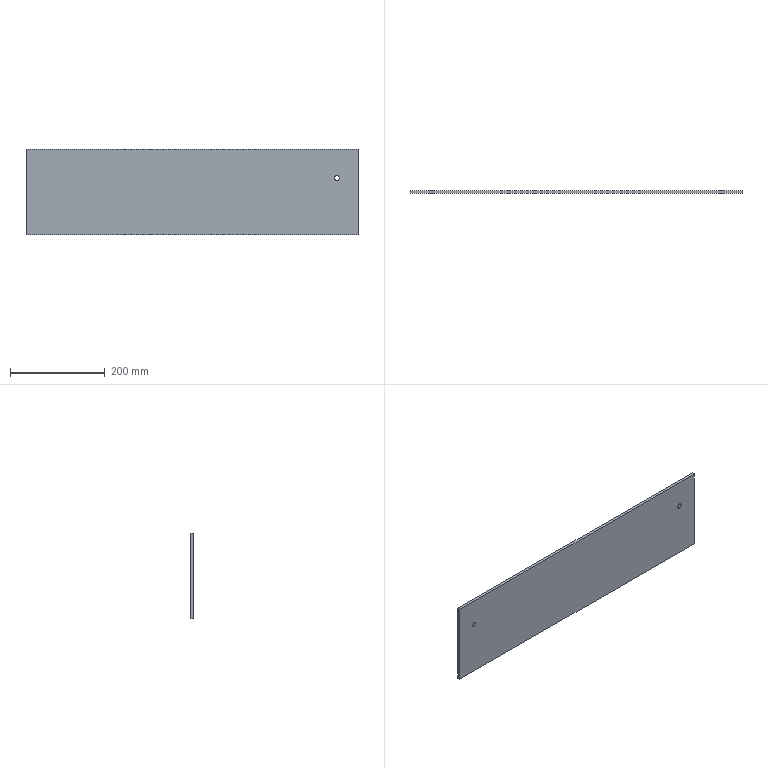Part | SolidWorks | features Cut 2, FlatPattern 1, SMBaseFlange 1, SheetMetal 1 | 1 solid | 11 faces | box 700 x 6 x 180 mm | volume 755105 mm3 | plane 7 | cylinder 4 | commonest cylinder face diameters 10 x4
STEP:
#1=CARTESIAN_POINT('',(48.5,-5.4,-60.5));
#2=VERTEX_POINT('',#1);
#3=CARTESIAN_POINT('',(38.5,-5.4,-60.5));
#4=VERTEX_POINT('',#3);
#5=CARTESIAN_POINT('',(43.5,-5.4,-60.5));
#6=DIRECTION('',(0.,1.,0.));
#7=DIRECTION('',(-1.,0.,0.));
#8=AXIS2_PLACEMENT_3D('',#5,#6,#7);
#9=CIRCLE('',#8,5.);
#10=EDGE_CURVE('',#2,#4,#9,.T.);
#11=ORIENTED_EDGE('',*,*,#10,.F.);
#12=CARTESIAN_POINT('',(48.5,0.,-60.5));
#13=VERTEX_POINT('',#12);
#14=CARTESIAN_POINT('',(48.5,-5.4,-60.5));
#15=DIRECTION('',(0.,1.,0.));
#16=VECTOR('',#15,1000.);
#17=LINE('',#14,#16);
#18=EDGE_CURVE('',#2,#13,#17,.T.);
#19=ORIENTED_EDGE('',*,*,#18,.T.);
#20=CARTESIAN_POINT('',(38.5,0.,-60.5));
#21=VERTEX_POINT('',#20);
#22=CARTESIAN_POINT('',(43.5,0.,-60.5));
#23=DIRECTION('',(0.,-1.,0.));
#24=DIRECTION('',(0.,0.,-1.));
#25=AXIS2_PLACEMENT_3D('',#22,#23,#24);
#26=CIRCLE('',#25,5.);
#27=EDGE_CURVE('',#21,#13,#26,.T.);
#28=ORIENTED_EDGE('',*,*,#27,.F.);
#29=CARTESIAN_POINT('',(38.5,-5.4,-60.5));
#30=DIRECTION('',(0.,1.,0.));
#31=VECTOR('',#30,1000.);
#32=LINE('',#29,#31);
#33=EDGE_CURVE('',#4,#21,#32,.T.);
#34=ORIENTED_EDGE('',*,*,#33,.F.);
#35=EDGE_LOOP('',(#11,#19,#28,#34));
#36=FACE_OUTER_BOUND('',#35,.T.);
#37=CARTESIAN_POINT('',(43.5,-5.4,-60.5));
#38=DIRECTION('',(0.,1.,0.));
#39=DIRECTION('',(-1.,0.,0.));
#40=AXIS2_PLACEMENT_3D('',#37,#38,#39);
#41=CYLINDRICAL_SURFACE('',#40,5.);
#42=ADVANCED_FACE('',(#36),#41,.F.);
#43=CARTESIAN_POINT('',(655.6,-6.,-55.5));
#44=VERTEX_POINT('',#43);
#45=CARTESIAN_POINT('',(655.6,-6.,-65.5));
#46=VERTEX_POINT('',#45);
#47=CARTESIAN_POINT('',(655.6,-6.,-60.5));
#48=DIRECTION('',(0.,-1.,0.));
#49=DIRECTION('',(0.,0.,-1.));
#50=AXIS2_PLACEMENT_3D('',#47,#48,#49);
#51=CIRCLE('',#50,5.);
#52=EDGE_CURVE('',#44,#46,#51,.T.);
#53=ORIENTED_EDGE('',*,*,#52,.T.);
#54=CARTESIAN_POINT('',(655.6,0.,-65.5));
#55=VERTEX_POINT('',#54);
#56=CARTESIAN_POINT('',(655.6,-9.9,-65.5));
#57=DIRECTION('',(0.,1.,0.));
#58=VECTOR('',#57,1000.);
#59=LINE('',#56,#58);
#60=EDGE_CURVE('',#46,#55,#59,.T.);
#61=ORIENTED_EDGE('',*,*,#60,.T.);
#62=CARTESIAN_POINT('',(655.6,0.,-55.5));
#63=VERTEX_POINT('',#62);
#64=CARTESIAN_POINT('',(655.6,0.,-60.5));
#65=DIRECTION('',(0.,-1.,0.));
#66=DIRECTION('',(0.,0.,-1.));
#67=AXIS2_PLACEMENT_3D('',#64,#65,#66);
#68=CIRCLE('',#67,5.);
#69=EDGE_CURVE('',#63,#55,#68,.T.);
#70=ORIENTED_EDGE('',*,*,#69,.F.);
#71=CARTESIAN_POINT('',(655.6,-9.9,-55.5));
#72=DIRECTION('',(0.,1.,0.));
#73=VECTOR('',#72,1000.);
#74=LINE('',#71,#73);
#75=EDGE_CURVE('',#44,#63,#74,.T.);
#76=ORIENTED_EDGE('',*,*,#75,.F.);
#77=EDGE_LOOP('',(#53,#61,#70,#76));
#78=FACE_OUTER_BOUND('',#77,.T.);
#79=CARTESIAN_POINT('',(655.6,-9.9,-60.5));
#80=DIRECTION('',(0.,1.,0.));
#81=DIRECTION('',(0.,0.,1.));
#82=AXIS2_PLACEMENT_3D('',#79,#80,#81);
#83=CYLINDRICAL_SURFACE('',#82,5.);
#84=ADVANCED_FACE('',(#78),#83,.F.);
#85=CARTESIAN_POINT('',(0.,0.,-180.));
#86=VERTEX_POINT('',#85);
#87=CARTESIAN_POINT('',(0.,0.,0.));
#88=VERTEX_POINT('',#87);
#89=CARTESIAN_POINT('',(0.,0.,0.));
#90=DIRECTION('',(0.,0.,1.));
#91=VECTOR('',#90,1000.);
#92=LINE('',#89,#91);
#93=EDGE_CURVE('',#86,#88,#92,.T.);
#94=ORIENTED_EDGE('',*,*,#93,.F.);
#95=CARTESIAN_POINT('',(0.,-6.,-180.));
#96=VERTEX_POINT('',#95);
#97=CARTESIAN_POINT('',(0.,-6.,-180.));
#98=DIRECTION('',(0.,1.,0.));
#99=VECTOR('',#98,1000.);
#100=LINE('',#97,#99);
#101=EDGE_CURVE('',#96,#86,#100,.T.);
#102=ORIENTED_EDGE('',*,*,#101,.F.);
#103=CARTESIAN_POINT('',(0.,-6.,0.));
#104=VERTEX_POINT('',#103);
#105=CARTESIAN_POINT('',(0.,-6.,0.));
#106=DIRECTION('',(0.,0.,1.));
#107=VECTOR('',#106,1000.);
#108=LINE('',#105,#107);
#109=EDGE_CURVE('',#96,#104,#108,.T.);
#110=ORIENTED_EDGE('',*,*,#109,.T.);
#111=CARTESIAN_POINT('',(0.,-6.,0.));
#112=DIRECTION('',(0.,1.,0.));
#113=VECTOR('',#112,1000.);
#114=LINE('',#111,#113);
#115=EDGE_CURVE('',#104,#88,#114,.T.);
#116=ORIENTED_EDGE('',*,*,#115,.T.);
#117=EDGE_LOOP('',(#94,#102,#110,#116));
#118=FACE_OUTER_BOUND('',#117,.T.);
#119=CARTESIAN_POINT('',(0.,-6.,0.));
#120=DIRECTION('',(-1.,0.,0.));
#121=DIRECTION('',(0.,0.,1.));
#122=AXIS2_PLACEMENT_3D('',#119,#120,#121);
#123=PLANE('',#122);
#124=ADVANCED_FACE('',(#118),#123,.T.);
#125=CARTESIAN_POINT('',(700.,0.,-180.));
#126=VERTEX_POINT('',#125);
#127=CARTESIAN_POINT('',(0.,0.,-180.));
#128=DIRECTION('',(-1.,0.,0.));
#129=VECTOR('',#128,1000.);
#130=LINE('',#127,#129);
#131=EDGE_CURVE('',#126,#86,#130,.T.);
#132=ORIENTED_EDGE('',*,*,#131,.F.);
#133=CARTESIAN_POINT('',(700.,-6.,-180.));
#134=VERTEX_POINT('',#133);
#135=CARTESIAN_POINT('',(700.,-6.,-180.));
#136=DIRECTION('',(0.,1.,0.));
#137=VECTOR('',#136,1000.);
#138=LINE('',#135,#137);
#139=EDGE_CURVE('',#134,#126,#138,.T.);
#140=ORIENTED_EDGE('',*,*,#139,.F.);
#141=CARTESIAN_POINT('',(0.,-6.,-180.));
#142=DIRECTION('',(-1.,0.,0.));
#143=VECTOR('',#142,1000.);
#144=LINE('',#141,#143);
#145=EDGE_CURVE('',#134,#96,#144,.T.);
#146=ORIENTED_EDGE('',*,*,#145,.T.);
#147=ORIENTED_EDGE('',*,*,#101,.T.);
#148=EDGE_LOOP('',(#132,#140,#146,#147));
#149=FACE_OUTER_BOUND('',#148,.T.);
#150=CARTESIAN_POINT('',(0.,-6.,-180.));
#151=DIRECTION('',(0.,0.,-1.));
#152=DIRECTION('',(-1.,0.,0.));
#153=AXIS2_PLACEMENT_3D('',#150,#151,#152);
#154=PLANE('',#153);
#155=ADVANCED_FACE('',(#149),#154,.T.);
#156=CARTESIAN_POINT('',(700.,0.,0.));
#157=VERTEX_POINT('',#156);
#158=CARTESIAN_POINT('',(700.,0.,0.));
#159=DIRECTION('',(0.,0.,-1.));
#160=VECTOR('',#159,1000.);
#161=LINE('',#158,#160);
#162=EDGE_CURVE('',#157,#126,#161,.T.);
#163=ORIENTED_EDGE('',*,*,#162,.F.);
#164=CARTESIAN_POINT('',(700.,-6.,0.));
#165=VERTEX_POINT('',#164);
#166=CARTESIAN_POINT('',(700.,-6.,0.));
#167=DIRECTION('',(0.,1.,0.));
#168=VECTOR('',#167,1000.);
#169=LINE('',#166,#168);
#170=EDGE_CURVE('',#165,#157,#169,.T.);
#171=ORIENTED_EDGE('',*,*,#170,.F.);
#172=CARTESIAN_POINT('',(700.,-6.,0.));
#173=DIRECTION('',(0.,0.,-1.));
#174=VECTOR('',#173,1000.);
#175=LINE('',#172,#174);
#176=EDGE_CURVE('',#165,#134,#175,.T.);
#177=ORIENTED_EDGE('',*,*,#176,.T.);
#178=ORIENTED_EDGE('',*,*,#139,.T.);
#179=EDGE_LOOP('',(#163,#171,#177,#178));
#180=FACE_OUTER_BOUND('',#179,.T.);
#181=CARTESIAN_POINT('',(700.,-6.,0.));
#182=DIRECTION('',(1.,0.,0.));
#183=DIRECTION('',(0.,0.,-1.));
#184=AXIS2_PLACEMENT_3D('',#181,#182,#183);
#185=PLANE('',#184);
#186=ADVANCED_FACE('',(#180),#185,.T.);
#187=CARTESIAN_POINT('',(0.,0.,0.));
#188=DIRECTION('',(1.,0.,0.));
#189=VECTOR('',#188,1000.);
#190=LINE('',#187,#189);
#191=EDGE_CURVE('',#88,#157,#190,.T.);
#192=ORIENTED_EDGE('',*,*,#191,.F.);
#193=ORIENTED_EDGE('',*,*,#115,.F.);
#194=CARTESIAN_POINT('',(0.,-6.,0.));
#195=DIRECTION('',(1.,0.,0.));
#196=VECTOR('',#195,1000.);
#197=LINE('',#194,#196);
#198=EDGE_CURVE('',#104,#165,#197,.T.);
#199=ORIENTED_EDGE('',*,*,#198,.T.);
#200=ORIENTED_EDGE('',*,*,#170,.T.);
#201=EDGE_LOOP('',(#192,#193,#199,#200));
#202=FACE_OUTER_BOUND('',#201,.T.);
#203=CARTESIAN_POINT('',(0.,-6.,0.));
#204=DIRECTION('',(0.,0.,1.));
#205=DIRECTION('',(1.,0.,0.));
#206=AXIS2_PLACEMENT_3D('',#203,#204,#205);
#207=PLANE('',#206);
#208=ADVANCED_FACE('',(#202),#207,.T.);
#209=ORIENTED_EDGE('',*,*,#52,.F.);
#210=CARTESIAN_POINT('',(655.6,-6.,-60.5));
#211=DIRECTION('',(0.,-1.,0.));
#212=DIRECTION('',(0.,0.,-1.));
#213=AXIS2_PLACEMENT_3D('',#210,#211,#212);
#214=CIRCLE('',#213,5.);
#215=EDGE_CURVE('',#46,#44,#214,.T.);
#216=ORIENTED_EDGE('',*,*,#215,.F.);
#217=EDGE_LOOP('',(#209,#216));
#218=FACE_BOUND('',#217,.T.);
#219=ORIENTED_EDGE('',*,*,#109,.F.);
#220=ORIENTED_EDGE('',*,*,#145,.F.);
#221=ORIENTED_EDGE('',*,*,#176,.F.);
#222=ORIENTED_EDGE('',*,*,#198,.F.);
#223=EDGE_LOOP('',(#219,#220,#221,#222));
#224=FACE_OUTER_BOUND('',#223,.T.);
#225=CARTESIAN_POINT('',(0.,-6.,0.));
#226=DIRECTION('',(0.,-1.,0.));
#227=DIRECTION('',(0.,0.,-1.));
#228=AXIS2_PLACEMENT_3D('',#225,#226,#227);
#229=PLANE('',#228);
#230=ADVANCED_FACE('',(#218,#224),#229,.T.);
#231=ORIENTED_EDGE('',*,*,#27,.T.);
#232=CARTESIAN_POINT('',(43.5,0.,-60.5));
#233=DIRECTION('',(0.,-1.,0.));
#234=DIRECTION('',(0.,0.,-1.));
#235=AXIS2_PLACEMENT_3D('',#232,#233,#234);
#236=CIRCLE('',#235,5.);
#237=EDGE_CURVE('',#13,#21,#236,.T.);
#238=ORIENTED_EDGE('',*,*,#237,.T.);
#239=EDGE_LOOP('',(#231,#238));
#240=FACE_BOUND('',#239,.T.);
#241=ORIENTED_EDGE('',*,*,#69,.T.);
#242=CARTESIAN_POINT('',(655.6,0.,-60.5));
#243=DIRECTION('',(0.,-1.,0.));
#244=DIRECTION('',(0.,0.,-1.));
#245=AXIS2_PLACEMENT_3D('',#242,#243,#244);
#246=CIRCLE('',#245,5.);
#247=EDGE_CURVE('',#55,#63,#246,.T.);
#248=ORIENTED_EDGE('',*,*,#247,.T.);
#249=EDGE_LOOP('',(#241,#248));
#250=FACE_BOUND('',#249,.T.);
#251=ORIENTED_EDGE('',*,*,#93,.T.);
#252=ORIENTED_EDGE('',*,*,#191,.T.);
#253=ORIENTED_EDGE('',*,*,#162,.T.);
#254=ORIENTED_EDGE('',*,*,#131,.T.);
#255=EDGE_LOOP('',(#251,#252,#253,#254));
#256=FACE_OUTER_BOUND('',#255,.T.);
#257=CARTESIAN_POINT('',(0.,0.,0.));
#258=DIRECTION('',(0.,-1.,0.));
#259=DIRECTION('',(0.,0.,-1.));
#260=AXIS2_PLACEMENT_3D('',#257,#258,#259);
#261=PLANE('',#260);
#262=ADVANCED_FACE('',(#240,#250,#256),#261,.F.);
#263=ORIENTED_EDGE('',*,*,#60,.F.);
#264=ORIENTED_EDGE('',*,*,#215,.T.);
#265=ORIENTED_EDGE('',*,*,#75,.T.);
#266=ORIENTED_EDGE('',*,*,#247,.F.);
#267=EDGE_LOOP('',(#263,#264,#265,#266));
#268=FACE_OUTER_BOUND('',#267,.T.);
#269=CARTESIAN_POINT('',(655.6,-9.9,-60.5));
#270=DIRECTION('',(0.,1.,0.));
#271=DIRECTION('',(0.,0.,1.));
#272=AXIS2_PLACEMENT_3D('',#269,#270,#271);
#273=CYLINDRICAL_SURFACE('',#272,5.);
#274=ADVANCED_FACE('',(#268),#273,.F.);
#275=ORIENTED_EDGE('',*,*,#18,.F.);
#276=CARTESIAN_POINT('',(43.5,-5.4,-60.5));
#277=DIRECTION('',(0.,1.,0.));
#278=DIRECTION('',(-1.,0.,0.));
#279=AXIS2_PLACEMENT_3D('',#276,#277,#278);
#280=CIRCLE('',#279,5.);
#281=EDGE_CURVE('',#4,#2,#280,.T.);
#282=ORIENTED_EDGE('',*,*,#281,.F.);
#283=ORIENTED_EDGE('',*,*,#33,.T.);
#284=ORIENTED_EDGE('',*,*,#237,.F.);
#285=EDGE_LOOP('',(#275,#282,#283,#284));
#286=FACE_OUTER_BOUND('',#285,.T.);
#287=CARTESIAN_POINT('',(43.5,-5.4,-60.5));
#288=DIRECTION('',(0.,1.,0.));
#289=DIRECTION('',(-1.,0.,0.));
#290=AXIS2_PLACEMENT_3D('',#287,#288,#289);
#291=CYLINDRICAL_SURFACE('',#290,5.);
#292=ADVANCED_FACE('',(#286),#291,.F.);
#293=ORIENTED_EDGE('',*,*,#281,.T.);
#294=ORIENTED_EDGE('',*,*,#10,.T.);
#295=EDGE_LOOP('',(#293,#294));
#296=FACE_OUTER_BOUND('',#295,.T.);
#297=CARTESIAN_POINT('',(43.5,-5.4,-60.5));
#298=DIRECTION('',(0.,1.,0.));
#299=DIRECTION('',(-1.,0.,0.));
#300=AXIS2_PLACEMENT_3D('',#297,#298,#299);
#301=PLANE('',#300);
#302=ADVANCED_FACE('',(#296),#301,.T.);
#303=CLOSED_SHELL('',(#42,#84,#124,#155,#186,#208,#230,#262,#274,#292,#302));
#304=MANIFOLD_SOLID_BREP('',#303);
#305=CARTESIAN_POINT('',(0.,0.,0.));
#306=DIRECTION('',(0.,0.,1.));
#307=DIRECTION('',(1.,0.,0.));
#308=AXIS2_PLACEMENT_3D('',#305,#306,#307);
#309=(LENGTH_UNIT()NAMED_UNIT(*)SI_UNIT(.MILLI.,.METRE.));
#310=UNCERTAINTY_MEASURE_WITH_UNIT(LENGTH_MEASURE(0.00001),#309,'','');
#311=(NAMED_UNIT(*)PLANE_ANGLE_UNIT()SI_UNIT($,.RADIAN.));
#312=(NAMED_UNIT(*)SI_UNIT($,.STERADIAN.)SOLID_ANGLE_UNIT());
#313=(GEOMETRIC_REPRESENTATION_CONTEXT(3)GLOBAL_UNCERTAINTY_ASSIGNED_CONTEXT((#310))GLOBAL_UNIT_ASSIGNED_CONTEXT((#309,#311,#312))REPRESENTATION_CONTEXT('',''));
#314=ADVANCED_BREP_SHAPE_REPRESENTATION('',(#304,#308),#313);